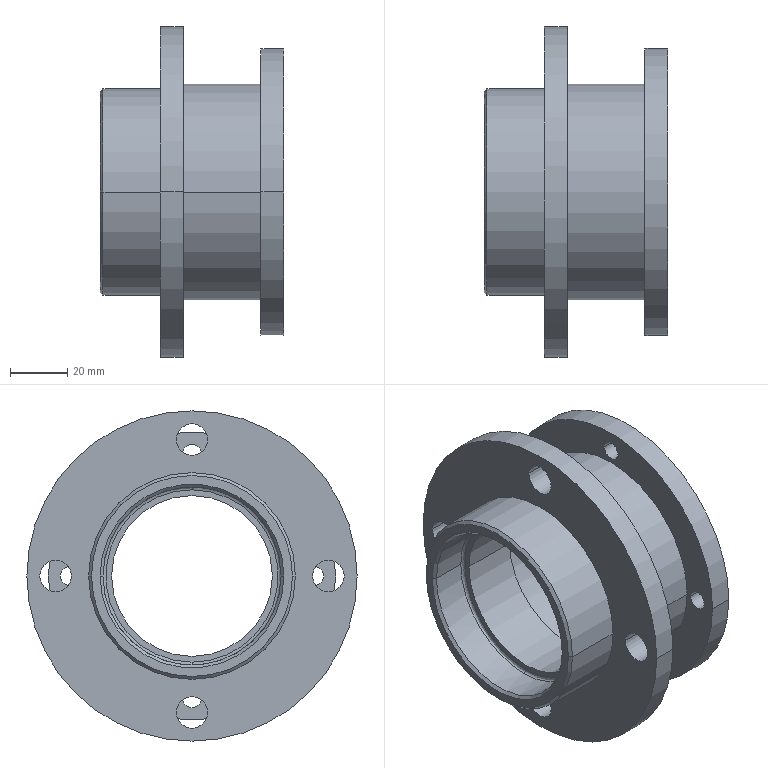Part | SolidWorks | features BaseBody 1 | 1 solid | 47 faces | box 64 x 115 x 115 mm | volume 164261 mm3 | cylinder 30 | plane 7 | cone 6 | spline 4 | commonest cylinder face diameters 6.647 x8 11 x8 62 x4 56 x2 72 x2 75 x2